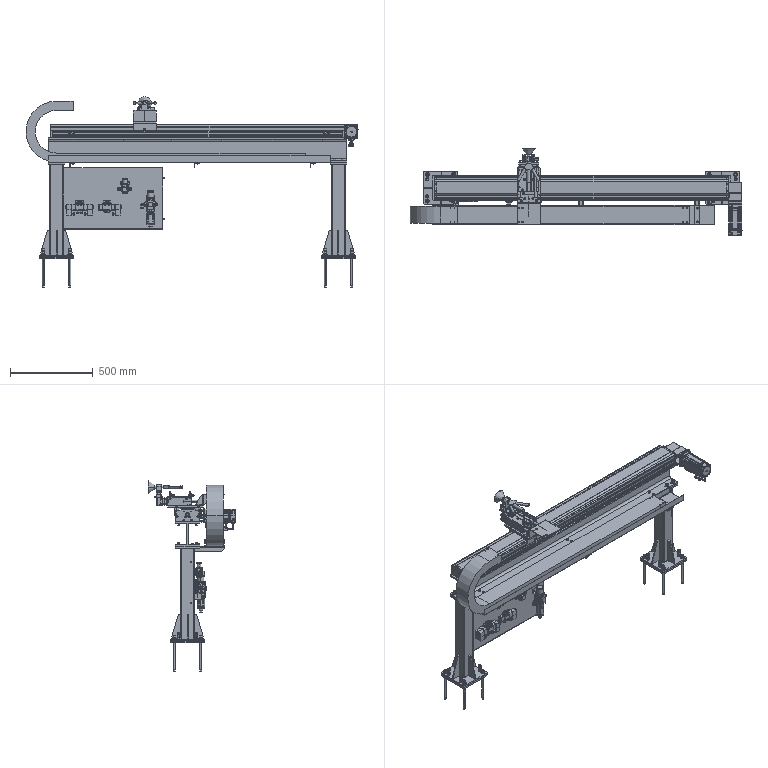Part | NX | features BREP 176 | 317 solids | 11044 faces | volume 26809605 mm3 | plane 4804 | cylinder 3616 | cone 1614 | torus 770 | spline 126 | sphere 114 | commonest cylinder face diameters 2 x260 6 x160 10 x154 1 x133 5 x130 3 x127